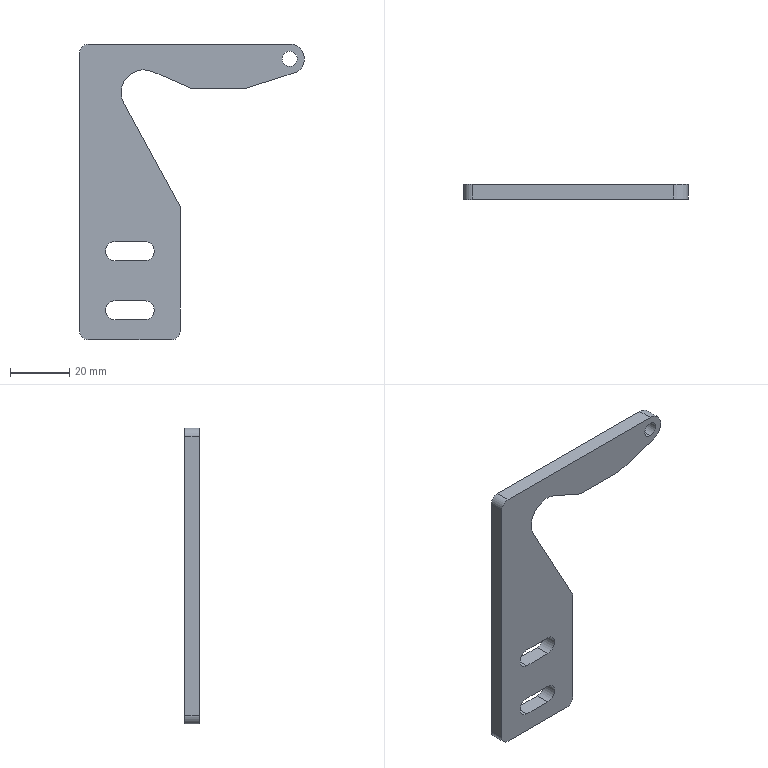Part | SolidWorks | features Extrusion 1, Fillet 1 | 1 solid | 25 faces | box 76 x 5 x 100 mm | volume 16067 mm3 | plane 14 | cylinder 11 | commonest cylinder face diameters 6.5 x4 6 x3 5.2 x2 10 x1 15.307 x1
STEP:
#1=CARTESIAN_POINT('',(54.,5.,82.4));
#2=VERTEX_POINT('',#1);
#3=CARTESIAN_POINT('',(54.,5.,87.6));
#4=VERTEX_POINT('',#3);
#5=CARTESIAN_POINT('',(54.,5.,85.));
#6=DIRECTION('',(0.,1.,0.));
#7=DIRECTION('',(0.,0.,1.));
#8=AXIS2_PLACEMENT_3D('',#5,#6,#7);
#9=CIRCLE('',#8,2.6);
#10=EDGE_CURVE('',#2,#4,#9,.T.);
#11=ORIENTED_EDGE('',*,*,#10,.T.);
#12=CARTESIAN_POINT('',(54.,0.,87.6));
#13=VERTEX_POINT('',#12);
#14=CARTESIAN_POINT('',(54.,5.,87.6));
#15=DIRECTION('',(0.,-1.,0.));
#16=VECTOR('',#15,1000.);
#17=LINE('',#14,#16);
#18=EDGE_CURVE('',#4,#13,#17,.T.);
#19=ORIENTED_EDGE('',*,*,#18,.T.);
#20=CARTESIAN_POINT('',(54.,0.,82.4));
#21=VERTEX_POINT('',#20);
#22=CARTESIAN_POINT('',(54.,0.,85.));
#23=DIRECTION('',(0.,1.,0.));
#24=DIRECTION('',(0.,0.,1.));
#25=AXIS2_PLACEMENT_3D('',#22,#23,#24);
#26=CIRCLE('',#25,2.6);
#27=EDGE_CURVE('',#21,#13,#26,.T.);
#28=ORIENTED_EDGE('',*,*,#27,.F.);
#29=CARTESIAN_POINT('',(54.,5.,82.4));
#30=DIRECTION('',(0.,-1.,0.));
#31=VECTOR('',#30,1000.);
#32=LINE('',#29,#31);
#33=EDGE_CURVE('',#2,#21,#32,.T.);
#34=ORIENTED_EDGE('',*,*,#33,.F.);
#35=EDGE_LOOP('',(#11,#19,#28,#34));
#36=FACE_OUTER_BOUND('',#35,.T.);
#37=CARTESIAN_POINT('',(54.,5.,85.));
#38=DIRECTION('',(0.,-1.,0.));
#39=DIRECTION('',(0.,0.,-1.));
#40=AXIS2_PLACEMENT_3D('',#37,#38,#39);
#41=CYLINDRICAL_SURFACE('',#40,2.6);
#42=ADVANCED_FACE('',(#36),#41,.F.);
#43=CARTESIAN_POINT('',(5.,5.,16.75));
#44=VERTEX_POINT('',#43);
#45=CARTESIAN_POINT('',(-5.,5.,16.75));
#46=VERTEX_POINT('',#45);
#47=CARTESIAN_POINT('',(5.,5.,16.75));
#48=DIRECTION('',(-1.,0.,0.));
#49=VECTOR('',#48,1000.);
#50=LINE('',#47,#49);
#51=EDGE_CURVE('',#44,#46,#50,.T.);
#52=ORIENTED_EDGE('',*,*,#51,.F.);
#53=CARTESIAN_POINT('',(5.,5.,23.25));
#54=VERTEX_POINT('',#53);
#55=CARTESIAN_POINT('',(5.,5.,20.));
#56=DIRECTION('',(0.,1.,0.));
#57=DIRECTION('',(0.,0.,1.));
#58=AXIS2_PLACEMENT_3D('',#55,#56,#57);
#59=CIRCLE('',#58,3.25);
#60=EDGE_CURVE('',#54,#44,#59,.T.);
#61=ORIENTED_EDGE('',*,*,#60,.F.);
#62=CARTESIAN_POINT('',(-5.,5.,23.25));
#63=VERTEX_POINT('',#62);
#64=CARTESIAN_POINT('',(5.,5.,23.25));
#65=DIRECTION('',(1.,0.,0.));
#66=VECTOR('',#65,1000.);
#67=LINE('',#64,#66);
#68=EDGE_CURVE('',#63,#54,#67,.T.);
#69=ORIENTED_EDGE('',*,*,#68,.F.);
#70=CARTESIAN_POINT('',(-5.,5.,20.));
#71=DIRECTION('',(0.,1.,0.));
#72=DIRECTION('',(0.,0.,1.));
#73=AXIS2_PLACEMENT_3D('',#70,#71,#72);
#74=CIRCLE('',#73,3.25);
#75=EDGE_CURVE('',#46,#63,#74,.T.);
#76=ORIENTED_EDGE('',*,*,#75,.F.);
#77=EDGE_LOOP('',(#52,#61,#69,#76));
#78=FACE_BOUND('',#77,.T.);
#79=CARTESIAN_POINT('',(5.,5.,-3.25));
#80=VERTEX_POINT('',#79);
#81=CARTESIAN_POINT('',(-5.,5.,-3.25));
#82=VERTEX_POINT('',#81);
#83=CARTESIAN_POINT('',(5.,5.,-3.25));
#84=DIRECTION('',(-1.,0.,0.));
#85=VECTOR('',#84,1000.);
#86=LINE('',#83,#85);
#87=EDGE_CURVE('',#80,#82,#86,.T.);
#88=ORIENTED_EDGE('',*,*,#87,.F.);
#89=CARTESIAN_POINT('',(5.,5.,3.25));
#90=VERTEX_POINT('',#89);
#91=CARTESIAN_POINT('',(5.,5.,0.));
#92=DIRECTION('',(0.,1.,0.));
#93=DIRECTION('',(0.,0.,1.));
#94=AXIS2_PLACEMENT_3D('',#91,#92,#93);
#95=CIRCLE('',#94,3.25);
#96=EDGE_CURVE('',#90,#80,#95,.T.);
#97=ORIENTED_EDGE('',*,*,#96,.F.);
#98=CARTESIAN_POINT('',(-5.,5.,3.25));
#99=VERTEX_POINT('',#98);
#100=CARTESIAN_POINT('',(5.,5.,3.25));
#101=DIRECTION('',(1.,0.,0.));
#102=VECTOR('',#101,1000.);
#103=LINE('',#100,#102);
#104=EDGE_CURVE('',#99,#90,#103,.T.);
#105=ORIENTED_EDGE('',*,*,#104,.F.);
#106=CARTESIAN_POINT('',(-5.,5.,0.));
#107=DIRECTION('',(0.,1.,0.));
#108=DIRECTION('',(0.,0.,1.));
#109=AXIS2_PLACEMENT_3D('',#106,#107,#108);
#110=CIRCLE('',#109,3.25);
#111=EDGE_CURVE('',#82,#99,#110,.T.);
#112=ORIENTED_EDGE('',*,*,#111,.F.);
#113=EDGE_LOOP('',(#88,#97,#105,#112));
#114=FACE_BOUND('',#113,.T.);
#115=CARTESIAN_POINT('',(14.,5.,-10.));
#116=VERTEX_POINT('',#115);
#117=CARTESIAN_POINT('',(-14.,5.,-10.));
#118=VERTEX_POINT('',#117);
#119=CARTESIAN_POINT('',(-17.,5.,-10.));
#120=DIRECTION('',(-1.,0.,0.));
#121=VECTOR('',#120,1000.);
#122=LINE('',#119,#121);
#123=EDGE_CURVE('',#116,#118,#122,.T.);
#124=ORIENTED_EDGE('',*,*,#123,.T.);
#125=CARTESIAN_POINT('',(-17.,5.,-7.));
#126=VERTEX_POINT('',#125);
#127=CARTESIAN_POINT('',(-14.,5.,-7.));
#128=DIRECTION('',(0.,1.,0.));
#129=DIRECTION('',(0.,0.,1.));
#130=AXIS2_PLACEMENT_3D('',#127,#128,#129);
#131=CIRCLE('',#130,3.);
#132=EDGE_CURVE('',#118,#126,#131,.T.);
#133=ORIENTED_EDGE('',*,*,#132,.T.);
#134=CARTESIAN_POINT('',(-17.,5.,87.));
#135=VERTEX_POINT('',#134);
#136=CARTESIAN_POINT('',(-17.,5.,-10.));
#137=DIRECTION('',(0.,0.,1.));
#138=VECTOR('',#137,1000.);
#139=LINE('',#136,#138);
#140=EDGE_CURVE('',#126,#135,#139,.T.);
#141=ORIENTED_EDGE('',*,*,#140,.T.);
#142=CARTESIAN_POINT('',(-14.,5.,90.));
#143=VERTEX_POINT('',#142);
#144=CARTESIAN_POINT('',(-14.,5.,87.));
#145=DIRECTION('',(0.,1.,0.));
#146=DIRECTION('',(0.,0.,1.));
#147=AXIS2_PLACEMENT_3D('',#144,#145,#146);
#148=CIRCLE('',#147,3.);
#149=EDGE_CURVE('',#135,#143,#148,.T.);
#150=ORIENTED_EDGE('',*,*,#149,.T.);
#151=CARTESIAN_POINT('',(54.,5.,90.));
#152=VERTEX_POINT('',#151);
#153=CARTESIAN_POINT('',(-17.,5.,90.));
#154=DIRECTION('',(1.,0.,0.));
#155=VECTOR('',#154,1000.);
#156=LINE('',#153,#155);
#157=EDGE_CURVE('',#143,#152,#156,.T.);
#158=ORIENTED_EDGE('',*,*,#157,.T.);
#159=CARTESIAN_POINT('',(55.511,5.,80.234));
#160=VERTEX_POINT('',#159);
#161=CARTESIAN_POINT('',(54.,5.,85.));
#162=DIRECTION('',(0.,1.,0.));
#163=DIRECTION('',(0.,0.,1.));
#164=AXIS2_PLACEMENT_3D('',#161,#162,#163);
#165=CIRCLE('',#164,5.);
#166=EDGE_CURVE('',#152,#160,#165,.T.);
#167=ORIENTED_EDGE('',*,*,#166,.T.);
#168=CARTESIAN_POINT('',(39.,5.,75.));
#169=VERTEX_POINT('',#168);
#170=CARTESIAN_POINT('',(39.,5.,75.));
#171=DIRECTION('',(-0.9533,0.,-0.3022));
#172=VECTOR('',#171,1000.);
#173=LINE('',#170,#172);
#174=EDGE_CURVE('',#160,#169,#173,.T.);
#175=ORIENTED_EDGE('',*,*,#174,.T.);
#176=CARTESIAN_POINT('',(20.726,5.,75.));
#177=VERTEX_POINT('',#176);
#178=CARTESIAN_POINT('',(39.,5.,75.));
#179=DIRECTION('',(-1.,0.,0.));
#180=VECTOR('',#179,1000.);
#181=LINE('',#178,#180);
#182=EDGE_CURVE('',#169,#177,#181,.T.);
#183=ORIENTED_EDGE('',*,*,#182,.T.);
#184=CARTESIAN_POINT('',(7.796,5.,80.662));
#185=VERTEX_POINT('',#184);
#186=CARTESIAN_POINT('',(20.726,5.,75.));
#187=DIRECTION('',(-0.916,0.,0.4011));
#188=VECTOR('',#187,1000.);
#189=LINE('',#186,#188);
#190=EDGE_CURVE('',#177,#185,#189,.T.);
#191=ORIENTED_EDGE('',*,*,#190,.T.);
#192=CARTESIAN_POINT('',(-2.,5.,70.));
#193=VERTEX_POINT('',#192);
#194=CARTESIAN_POINT('',(4.726,5.,73.651));
#195=DIRECTION('',(0.,-1.,0.));
#196=DIRECTION('',(0.,0.,1.));
#197=AXIS2_PLACEMENT_3D('',#194,#195,#196);
#198=CIRCLE('',#197,7.653);
#199=EDGE_CURVE('',#185,#193,#198,.T.);
#200=ORIENTED_EDGE('',*,*,#199,.T.);
#201=CARTESIAN_POINT('',(17.,5.,35.));
#202=VERTEX_POINT('',#201);
#203=CARTESIAN_POINT('',(17.,5.,35.));
#204=DIRECTION('',(0.4771,0.,-0.8789));
#205=VECTOR('',#204,1000.);
#206=LINE('',#203,#205);
#207=EDGE_CURVE('',#193,#202,#206,.T.);
#208=ORIENTED_EDGE('',*,*,#207,.T.);
#209=CARTESIAN_POINT('',(17.,5.,-7.));
#210=VERTEX_POINT('',#209);
#211=CARTESIAN_POINT('',(17.,5.,-10.));
#212=DIRECTION('',(0.,0.,-1.));
#213=VECTOR('',#212,1000.);
#214=LINE('',#211,#213);
#215=EDGE_CURVE('',#202,#210,#214,.T.);
#216=ORIENTED_EDGE('',*,*,#215,.T.);
#217=CARTESIAN_POINT('',(14.,5.,-7.));
#218=DIRECTION('',(0.,1.,0.));
#219=DIRECTION('',(0.,0.,1.));
#220=AXIS2_PLACEMENT_3D('',#217,#218,#219);
#221=CIRCLE('',#220,3.);
#222=EDGE_CURVE('',#210,#116,#221,.T.);
#223=ORIENTED_EDGE('',*,*,#222,.T.);
#224=EDGE_LOOP('',(#124,#133,#141,#150,#158,#167,#175,#183,#191,#200,#208,#216,#223));
#225=FACE_OUTER_BOUND('',#224,.T.);
#226=ORIENTED_EDGE('',*,*,#10,.F.);
#227=CARTESIAN_POINT('',(54.,5.,85.));
#228=DIRECTION('',(0.,1.,0.));
#229=DIRECTION('',(0.,0.,1.));
#230=AXIS2_PLACEMENT_3D('',#227,#228,#229);
#231=CIRCLE('',#230,2.6);
#232=EDGE_CURVE('',#4,#2,#231,.T.);
#233=ORIENTED_EDGE('',*,*,#232,.F.);
#234=EDGE_LOOP('',(#226,#233));
#235=FACE_BOUND('',#234,.T.);
#236=CARTESIAN_POINT('',(4.726,5.,73.651));
#237=DIRECTION('',(0.,1.,0.));
#238=DIRECTION('',(0.,0.,1.));
#239=AXIS2_PLACEMENT_3D('',#236,#237,#238);
#240=PLANE('',#239);
#241=ADVANCED_FACE('',(#78,#114,#225,#235),#240,.T.);
#242=CARTESIAN_POINT('',(5.,0.,3.25));
#243=VERTEX_POINT('',#242);
#244=CARTESIAN_POINT('',(5.,0.,-3.25));
#245=VERTEX_POINT('',#244);
#246=CARTESIAN_POINT('',(5.,0.,0.));
#247=DIRECTION('',(0.,1.,0.));
#248=DIRECTION('',(0.,0.,1.));
#249=AXIS2_PLACEMENT_3D('',#246,#247,#248);
#250=CIRCLE('',#249,3.25);
#251=EDGE_CURVE('',#243,#245,#250,.T.);
#252=ORIENTED_EDGE('',*,*,#251,.T.);
#253=CARTESIAN_POINT('',(-5.,0.,-3.25));
#254=VERTEX_POINT('',#253);
#255=CARTESIAN_POINT('',(5.,0.,-3.25));
#256=DIRECTION('',(-1.,0.,0.));
#257=VECTOR('',#256,1000.);
#258=LINE('',#255,#257);
#259=EDGE_CURVE('',#245,#254,#258,.T.);
#260=ORIENTED_EDGE('',*,*,#259,.T.);
#261=CARTESIAN_POINT('',(-5.,0.,3.25));
#262=VERTEX_POINT('',#261);
#263=CARTESIAN_POINT('',(-5.,0.,0.));
#264=DIRECTION('',(0.,1.,0.));
#265=DIRECTION('',(0.,0.,1.));
#266=AXIS2_PLACEMENT_3D('',#263,#264,#265);
#267=CIRCLE('',#266,3.25);
#268=EDGE_CURVE('',#254,#262,#267,.T.);
#269=ORIENTED_EDGE('',*,*,#268,.T.);
#270=CARTESIAN_POINT('',(5.,0.,3.25));
#271=DIRECTION('',(1.,0.,0.));
#272=VECTOR('',#271,1000.);
#273=LINE('',#270,#272);
#274=EDGE_CURVE('',#262,#243,#273,.T.);
#275=ORIENTED_EDGE('',*,*,#274,.T.);
#276=EDGE_LOOP('',(#252,#260,#269,#275));
#277=FACE_BOUND('',#276,.T.);
#278=CARTESIAN_POINT('',(-17.,0.,-7.));
#279=VERTEX_POINT('',#278);
#280=CARTESIAN_POINT('',(-17.,0.,87.));
#281=VERTEX_POINT('',#280);
#282=CARTESIAN_POINT('',(-17.,0.,-10.));
#283=DIRECTION('',(0.,0.,1.));
#284=VECTOR('',#283,1000.);
#285=LINE('',#282,#284);
#286=EDGE_CURVE('',#279,#281,#285,.T.);
#287=ORIENTED_EDGE('',*,*,#286,.F.);
#288=CARTESIAN_POINT('',(-14.,0.,-10.));
#289=VERTEX_POINT('',#288);
#290=CARTESIAN_POINT('',(-14.,0.,-7.));
#291=DIRECTION('',(0.,-1.,0.));
#292=DIRECTION('',(0.,0.,1.));
#293=AXIS2_PLACEMENT_3D('',#290,#291,#292);
#294=CIRCLE('',#293,3.);
#295=EDGE_CURVE('',#279,#289,#294,.T.);
#296=ORIENTED_EDGE('',*,*,#295,.T.);
#297=CARTESIAN_POINT('',(14.,0.,-10.));
#298=VERTEX_POINT('',#297);
#299=CARTESIAN_POINT('',(-17.,0.,-10.));
#300=DIRECTION('',(-1.,0.,0.));
#301=VECTOR('',#300,1000.);
#302=LINE('',#299,#301);
#303=EDGE_CURVE('',#298,#289,#302,.T.);
#304=ORIENTED_EDGE('',*,*,#303,.F.);
#305=CARTESIAN_POINT('',(17.,0.,-7.));
#306=VERTEX_POINT('',#305);
#307=CARTESIAN_POINT('',(14.,0.,-7.));
#308=DIRECTION('',(0.,-1.,0.));
#309=DIRECTION('',(0.,0.,1.));
#310=AXIS2_PLACEMENT_3D('',#307,#308,#309);
#311=CIRCLE('',#310,3.);
#312=EDGE_CURVE('',#298,#306,#311,.T.);
#313=ORIENTED_EDGE('',*,*,#312,.T.);
#314=CARTESIAN_POINT('',(17.,0.,35.));
#315=VERTEX_POINT('',#314);
#316=CARTESIAN_POINT('',(17.,0.,-10.));
#317=DIRECTION('',(0.,0.,-1.));
#318=VECTOR('',#317,1000.);
#319=LINE('',#316,#318);
#320=EDGE_CURVE('',#315,#306,#319,.T.);
#321=ORIENTED_EDGE('',*,*,#320,.F.);
#322=CARTESIAN_POINT('',(-2.,0.,70.));
#323=VERTEX_POINT('',#322);
#324=CARTESIAN_POINT('',(17.,0.,35.));
#325=DIRECTION('',(0.4771,0.,-0.8789));
#326=VECTOR('',#325,1000.);
#327=LINE('',#324,#326);
#328=EDGE_CURVE('',#323,#315,#327,.T.);
#329=ORIENTED_EDGE('',*,*,#328,.F.);
#330=CARTESIAN_POINT('',(7.796,0.,80.662));
#331=VERTEX_POINT('',#330);
#332=CARTESIAN_POINT('',(4.726,0.,73.651));
#333=DIRECTION('',(0.,-1.,0.));
#334=DIRECTION('',(0.,0.,1.));
#335=AXIS2_PLACEMENT_3D('',#332,#333,#334);
#336=CIRCLE('',#335,7.653);
#337=EDGE_CURVE('',#331,#323,#336,.T.);
#338=ORIENTED_EDGE('',*,*,#337,.F.);
#339=CARTESIAN_POINT('',(20.726,0.,75.));
#340=VERTEX_POINT('',#339);
#341=CARTESIAN_POINT('',(20.726,0.,75.));
#342=DIRECTION('',(-0.916,0.,0.4011));
#343=VECTOR('',#342,1000.);
#344=LINE('',#341,#343);
#345=EDGE_CURVE('',#340,#331,#344,.T.);
#346=ORIENTED_EDGE('',*,*,#345,.F.);
#347=CARTESIAN_POINT('',(39.,0.,75.));
#348=VERTEX_POINT('',#347);
#349=CARTESIAN_POINT('',(39.,0.,75.));
#350=DIRECTION('',(-1.,0.,0.));
#351=VECTOR('',#350,1000.);
#352=LINE('',#349,#351);
#353=EDGE_CURVE('',#348,#340,#352,.T.);
#354=ORIENTED_EDGE('',*,*,#353,.F.);
#355=CARTESIAN_POINT('',(55.511,0.,80.234));
#356=VERTEX_POINT('',#355);
#357=CARTESIAN_POINT('',(39.,0.,75.));
#358=DIRECTION('',(-0.9533,0.,-0.3022));
#359=VECTOR('',#358,1000.);
#360=LINE('',#357,#359);
#361=EDGE_CURVE('',#356,#348,#360,.T.);
#362=ORIENTED_EDGE('',*,*,#361,.F.);
#363=CARTESIAN_POINT('',(54.,0.,90.));
#364=VERTEX_POINT('',#363);
#365=CARTESIAN_POINT('',(54.,0.,85.));
#366=DIRECTION('',(0.,1.,0.));
#367=DIRECTION('',(0.,0.,1.));
#368=AXIS2_PLACEMENT_3D('',#365,#366,#367);
#369=CIRCLE('',#368,5.);
#370=EDGE_CURVE('',#364,#356,#369,.T.);
#371=ORIENTED_EDGE('',*,*,#370,.F.);
#372=CARTESIAN_POINT('',(-14.,0.,90.));
#373=VERTEX_POINT('',#372);
#374=CARTESIAN_POINT('',(-17.,0.,90.));
#375=DIRECTION('',(1.,0.,0.));
#376=VECTOR('',#375,1000.);
#377=LINE('',#374,#376);
#378=EDGE_CURVE('',#373,#364,#377,.T.);
#379=ORIENTED_EDGE('',*,*,#378,.F.);
#380=CARTESIAN_POINT('',(-14.,0.,87.));
#381=DIRECTION('',(0.,-1.,0.));
#382=DIRECTION('',(0.,0.,1.));
#383=AXIS2_PLACEMENT_3D('',#380,#381,#382);
#384=CIRCLE('',#383,3.);
#385=EDGE_CURVE('',#373,#281,#384,.T.);
#386=ORIENTED_EDGE('',*,*,#385,.T.);
#387=EDGE_LOOP('',(#287,#296,#304,#313,#321,#329,#338,#346,#354,#362,#371,#379,#386));
#388=FACE_OUTER_BOUND('',#387,.T.);
#389=CARTESIAN_POINT('',(5.,0.,23.25));
#390=VERTEX_POINT('',#389);
#391=CARTESIAN_POINT('',(5.,0.,16.75));
#392=VERTEX_POINT('',#391);
#393=CARTESIAN_POINT('',(5.,0.,20.));
#394=DIRECTION('',(0.,1.,0.));
#395=DIRECTION('',(0.,0.,1.));
#396=AXIS2_PLACEMENT_3D('',#393,#394,#395);
#397=CIRCLE('',#396,3.25);
#398=EDGE_CURVE('',#390,#392,#397,.T.);
#399=ORIENTED_EDGE('',*,*,#398,.T.);
#400=CARTESIAN_POINT('',(-5.,0.,16.75));
#401=VERTEX_POINT('',#400);
#402=CARTESIAN_POINT('',(5.,0.,16.75));
#403=DIRECTION('',(-1.,0.,0.));
#404=VECTOR('',#403,1000.);
#405=LINE('',#402,#404);
#406=EDGE_CURVE('',#392,#401,#405,.T.);
#407=ORIENTED_EDGE('',*,*,#406,.T.);
#408=CARTESIAN_POINT('',(-5.,0.,23.25));
#409=VERTEX_POINT('',#408);
#410=CARTESIAN_POINT('',(-5.,0.,20.));
#411=DIRECTION('',(0.,1.,0.));
#412=DIRECTION('',(0.,0.,1.));
#413=AXIS2_PLACEMENT_3D('',#410,#411,#412);
#414=CIRCLE('',#413,3.25);
#415=EDGE_CURVE('',#401,#409,#414,.T.);
#416=ORIENTED_EDGE('',*,*,#415,.T.);
#417=CARTESIAN_POINT('',(5.,0.,23.25));
#418=DIRECTION('',(1.,0.,0.));
#419=VECTOR('',#418,1000.);
#420=LINE('',#417,#419);
#421=EDGE_CURVE('',#409,#390,#420,.T.);
#422=ORIENTED_EDGE('',*,*,#421,.T.);
#423=EDGE_LOOP('',(#399,#407,#416,#422));
#424=FACE_BOUND('',#423,.T.);
#425=ORIENTED_EDGE('',*,*,#27,.T.);
#426=CARTESIAN_POINT('',(54.,0.,85.));
#427=DIRECTION('',(0.,1.,0.));
#428=DIRECTION('',(0.,0.,1.));
#429=AXIS2_PLACEMENT_3D('',#426,#427,#428);
#430=CIRCLE('',#429,2.6);
#431=EDGE_CURVE('',#13,#21,#430,.T.);
#432=ORIENTED_EDGE('',*,*,#431,.T.);
#433=EDGE_LOOP('',(#425,#432));
#434=FACE_BOUND('',#433,.T.);
#435=CARTESIAN_POINT('',(4.726,0.,73.651));
#436=DIRECTION('',(0.,1.,0.));
#437=DIRECTION('',(0.,0.,1.));
#438=AXIS2_PLACEMENT_3D('',#435,#436,#437);
#439=PLANE('',#438);
#440=ADVANCED_FACE('',(#277,#388,#424,#434),#439,.F.);
#441=ORIENTED_EDGE('',*,*,#303,.T.);
#442=CARTESIAN_POINT('',(-14.,5.,-10.));
#443=DIRECTION('',(0.,1.,0.));
#444=VECTOR('',#443,1000.);
#445=LINE('',#442,#444);
#446=EDGE_CURVE('',#289,#118,#445,.T.);
#447=ORIENTED_EDGE('',*,*,#446,.T.);
#448=ORIENTED_EDGE('',*,*,#123,.F.);
#449=CARTESIAN_POINT('',(14.,5.,-10.));
#450=DIRECTION('',(0.,-1.,0.));
#451=VECTOR('',#450,1000.);
#452=LINE('',#449,#451);
#453=EDGE_CURVE('',#116,#298,#452,.T.);
#454=ORIENTED_EDGE('',*,*,#453,.T.);
#455=EDGE_LOOP('',(#441,#447,#448,#454));
#456=FACE_OUTER_BOUND('',#455,.T.);
#457=CARTESIAN_POINT('',(-17.,5.,-10.));
#458=DIRECTION('',(0.,0.,1.));
#459=DIRECTION('',(1.,0.,0.));
#460=AXIS2_PLACEMENT_3D('',#457,#458,#459);
#461=PLANE('',#460);
#462=ADVANCED_FACE('',(#456),#461,.F.);
#463=ORIENTED_EDGE('',*,*,#140,.F.);
#464=CARTESIAN_POINT('',(-17.,5.,-7.));
#465=DIRECTION('',(0.,-1.,0.));
#466=VECTOR('',#465,1000.);
#467=LINE('',#464,#466);
#468=EDGE_CURVE('',#126,#279,#467,.T.);
#469=ORIENTED_EDGE('',*,*,#468,.T.);
#470=ORIENTED_EDGE('',*,*,#286,.T.);
#471=CARTESIAN_POINT('',(-17.,5.,87.));
#472=DIRECTION('',(0.,1.,0.));
#473=VECTOR('',#472,1000.);
#474=LINE('',#471,#473);
#475=EDGE_CURVE('',#281,#135,#474,.T.);
#476=ORIENTED_EDGE('',*,*,#475,.T.);
#477=EDGE_LOOP('',(#463,#469,#470,#476));
#478=FACE_OUTER_BOUND('',#477,.T.);
#479=CARTESIAN_POINT('',(-17.,5.,-10.));
#480=DIRECTION('',(1.,0.,0.));
#481=DIRECTION('',(0.,0.,-1.));
#482=AXIS2_PLACEMENT_3D('',#479,#480,#481);
#483=PLANE('',#482);
#484=ADVANCED_FACE('',(#478),#483,.F.);
#485=ORIENTED_EDGE('',*,*,#157,.F.);
#486=CARTESIAN_POINT('',(-14.,5.,90.));
#487=DIRECTION('',(0.,-1.,0.));
#488=VECTOR('',#487,1000.);
#489=LINE('',#486,#488);
#490=EDGE_CURVE('',#143,#373,#489,.T.);
#491=ORIENTED_EDGE('',*,*,#490,.T.);
#492=ORIENTED_EDGE('',*,*,#378,.T.);
#493=CARTESIAN_POINT('',(54.,5.,90.));
#494=DIRECTION('',(0.,-1.,0.));
#495=VECTOR('',#494,1000.);
#496=LINE('',#493,#495);
#497=EDGE_CURVE('',#152,#364,#496,.T.);
#498=ORIENTED_EDGE('',*,*,#497,.F.);
#499=EDGE_LOOP('',(#485,#491,#492,#498));
#500=FACE_OUTER_BOUND('',#499,.T.);
#501=CARTESIAN_POINT('',(-17.,5.,90.));
#502=DIRECTION('',(0.,0.,-1.));
#503=DIRECTION('',(-1.,0.,0.));
#504=AXIS2_PLACEMENT_3D('',#501,#502,#503);
#505=PLANE('',#504);
#506=ADVANCED_FACE('',(#500),#505,.F.);
#507=ORIENTED_EDGE('',*,*,#370,.T.);
#508=CARTESIAN_POINT('',(55.511,5.,80.234));
#509=DIRECTION('',(0.,-1.,0.));
#510=VECTOR('',#509,1000.);
#511=LINE('',#508,#510);
#512=EDGE_CURVE('',#160,#356,#511,.T.);
#513=ORIENTED_EDGE('',*,*,#512,.F.);
#514=ORIENTED_EDGE('',*,*,#166,.F.);
#515=ORIENTED_EDGE('',*,*,#497,.T.);
#516=EDGE_LOOP('',(#507,#513,#514,#515));
#517=FACE_OUTER_BOUND('',#516,.T.);
#518=CARTESIAN_POINT('',(54.,5.,85.));
#519=DIRECTION('',(0.,-1.,0.));
#520=DIRECTION('',(0.,0.,-1.));
#521=AXIS2_PLACEMENT_3D('',#518,#519,#520);
#522=CYLINDRICAL_SURFACE('',#521,5.);
#523=ADVANCED_FACE('',(#517),#522,.T.);
#524=ORIENTED_EDGE('',*,*,#361,.T.);
#525=CARTESIAN_POINT('',(39.,5.,75.));
#526=DIRECTION('',(0.,-1.,0.));
#527=VECTOR('',#526,1000.);
#528=LINE('',#525,#527);
#529=EDGE_CURVE('',#169,#348,#528,.T.);
#530=ORIENTED_EDGE('',*,*,#529,.F.);
#531=ORIENTED_EDGE('',*,*,#174,.F.);
#532=ORIENTED_EDGE('',*,*,#512,.T.);
#533=EDGE_LOOP('',(#524,#530,#531,#532));
#534=FACE_OUTER_BOUND('',#533,.T.);
#535=CARTESIAN_POINT('',(39.,5.,75.));
#536=DIRECTION('',(-0.3022,0.,0.9533));
#537=DIRECTION('',(0.9533,0.,0.3022));
#538=AXIS2_PLACEMENT_3D('',#535,#536,#537);
#539=PLANE('',#538);
#540=ADVANCED_FACE('',(#534),#539,.F.);
#541=ORIENTED_EDGE('',*,*,#353,.T.);
#542=CARTESIAN_POINT('',(20.726,5.,75.));
#543=DIRECTION('',(0.,-1.,0.));
#544=VECTOR('',#543,1000.);
#545=LINE('',#542,#544);
#546=EDGE_CURVE('',#177,#340,#545,.T.);
#547=ORIENTED_EDGE('',*,*,#546,.F.);
#548=ORIENTED_EDGE('',*,*,#182,.F.);
#549=ORIENTED_EDGE('',*,*,#529,.T.);
#550=EDGE_LOOP('',(#541,#547,#548,#549));
#551=FACE_OUTER_BOUND('',#550,.T.);
#552=CARTESIAN_POINT('',(39.,5.,75.));
#553=DIRECTION('',(0.,0.,1.));
#554=DIRECTION('',(1.,0.,0.));
#555=AXIS2_PLACEMENT_3D('',#552,#553,#554);
#556=PLANE('',#555);
#557=ADVANCED_FACE('',(#551),#556,.F.);
#558=ORIENTED_EDGE('',*,*,#345,.T.);
#559=CARTESIAN_POINT('',(7.796,5.,80.662));
#560=DIRECTION('',(0.,-1.,0.));
#561=VECTOR('',#560,1000.);
#562=LINE('',#559,#561);
#563=EDGE_CURVE('',#185,#331,#562,.T.);
#564=ORIENTED_EDGE('',*,*,#563,.F.);
#565=ORIENTED_EDGE('',*,*,#190,.F.);
#566=ORIENTED_EDGE('',*,*,#546,.T.);
#567=EDGE_LOOP('',(#558,#564,#565,#566));
#568=FACE_OUTER_BOUND('',#567,.T.);
#569=CARTESIAN_POINT('',(20.726,5.,75.));
#570=DIRECTION('',(0.4011,0.,0.916));
#571=DIRECTION('',(0.916,0.,-0.4011));
#572=AXIS2_PLACEMENT_3D('',#569,#570,#571);
#573=PLANE('',#572);
#574=ADVANCED_FACE('',(#568),#573,.F.);
#575=ORIENTED_EDGE('',*,*,#337,.T.);
#576=CARTESIAN_POINT('',(-2.,5.,70.));
#577=DIRECTION('',(0.,-1.,0.));
#578=VECTOR('',#577,1000.);
#579=LINE('',#576,#578);
#580=EDGE_CURVE('',#193,#323,#579,.T.);
#581=ORIENTED_EDGE('',*,*,#580,.F.);
#582=ORIENTED_EDGE('',*,*,#199,.F.);
#583=ORIENTED_EDGE('',*,*,#563,.T.);
#584=EDGE_LOOP('',(#575,#581,#582,#583));
#585=FACE_OUTER_BOUND('',#584,.T.);
#586=CARTESIAN_POINT('',(4.726,5.,73.651));
#587=DIRECTION('',(0.,-1.,0.));
#588=DIRECTION('',(0.,0.,-1.));
#589=AXIS2_PLACEMENT_3D('',#586,#587,#588);
#590=CYLINDRICAL_SURFACE('',#589,7.653);
#591=ADVANCED_FACE('',(#585),#590,.F.);
#592=ORIENTED_EDGE('',*,*,#328,.T.);
#593=CARTESIAN_POINT('',(17.,5.,35.));
#594=DIRECTION('',(0.,-1.,0.));
#595=VECTOR('',#594,1000.);
#596=LINE('',#593,#595);
#597=EDGE_CURVE('',#202,#315,#596,.T.);
#598=ORIENTED_EDGE('',*,*,#597,.F.);
#599=ORIENTED_EDGE('',*,*,#207,.F.);
#600=ORIENTED_EDGE('',*,*,#580,.T.);
#601=EDGE_LOOP('',(#592,#598,#599,#600));
#602=FACE_OUTER_BOUND('',#601,.T.);
#603=CARTESIAN_POINT('',(17.,5.,35.));
#604=DIRECTION('',(-0.8789,0.,-0.4771));
#605=DIRECTION('',(-0.4771,0.,0.8789));
#606=AXIS2_PLACEMENT_3D('',#603,#604,#605);
#607=PLANE('',#606);
#608=ADVANCED_FACE('',(#602),#607,.F.);
#609=ORIENTED_EDGE('',*,*,#320,.T.);
#610=CARTESIAN_POINT('',(17.,5.,-7.));
#611=DIRECTION('',(0.,1.,0.));
#612=VECTOR('',#611,1000.);
#613=LINE('',#610,#612);
#614=EDGE_CURVE('',#306,#210,#613,.T.);
#615=ORIENTED_EDGE('',*,*,#614,.T.);
#616=ORIENTED_EDGE('',*,*,#215,.F.);
#617=ORIENTED_EDGE('',*,*,#597,.T.);
#618=EDGE_LOOP('',(#609,#615,#616,#617));
#619=FACE_OUTER_BOUND('',#618,.T.);
#620=CARTESIAN_POINT('',(17.,5.,-10.));
#621=DIRECTION('',(-1.,0.,0.));
#622=DIRECTION('',(0.,0.,1.));
#623=AXIS2_PLACEMENT_3D('',#620,#621,#622);
#624=PLANE('',#623);
#625=ADVANCED_FACE('',(#619),#624,.F.);
#626=ORIENTED_EDGE('',*,*,#251,.F.);
#627=CARTESIAN_POINT('',(5.,5.,3.25));
#628=DIRECTION('',(0.,-1.,0.));
#629=VECTOR('',#628,1000.);
#630=LINE('',#627,#629);
#631=EDGE_CURVE('',#90,#243,#630,.T.);
#632=ORIENTED_EDGE('',*,*,#631,.F.);
#633=ORIENTED_EDGE('',*,*,#96,.T.);
#634=CARTESIAN_POINT('',(5.,5.,-3.25));
#635=DIRECTION('',(0.,-1.,0.));
#636=VECTOR('',#635,1000.);
#637=LINE('',#634,#636);
#638=EDGE_CURVE('',#80,#245,#637,.T.);
#639=ORIENTED_EDGE('',*,*,#638,.T.);
#640=EDGE_LOOP('',(#626,#632,#633,#639));
#641=FACE_OUTER_BOUND('',#640,.T.);
#642=CARTESIAN_POINT('',(5.,5.,0.));
#643=DIRECTION('',(0.,-1.,0.));
#644=DIRECTION('',(0.,0.,-1.));
#645=AXIS2_PLACEMENT_3D('',#642,#643,#644);
#646=CYLINDRICAL_SURFACE('',#645,3.25);
#647=ADVANCED_FACE('',(#641),#646,.F.);
#648=ORIENTED_EDGE('',*,*,#259,.F.);
#649=ORIENTED_EDGE('',*,*,#638,.F.);
#650=ORIENTED_EDGE('',*,*,#87,.T.);
#651=CARTESIAN_POINT('',(-5.,5.,-3.25));
#652=DIRECTION('',(0.,-1.,0.));
#653=VECTOR('',#652,1000.);
#654=LINE('',#651,#653);
#655=EDGE_CURVE('',#82,#254,#654,.T.);
#656=ORIENTED_EDGE('',*,*,#655,.T.);
#657=EDGE_LOOP('',(#648,#649,#650,#656));
#658=FACE_OUTER_BOUND('',#657,.T.);
#659=CARTESIAN_POINT('',(5.,5.,-3.25));
#660=DIRECTION('',(0.,0.,1.));
#661=DIRECTION('',(1.,0.,0.));
#662=AXIS2_PLACEMENT_3D('',#659,#660,#661);
#663=PLANE('',#662);
#664=ADVANCED_FACE('',(#658),#663,.T.);
#665=ORIENTED_EDGE('',*,*,#268,.F.);
#666=ORIENTED_EDGE('',*,*,#655,.F.);
#667=ORIENTED_EDGE('',*,*,#111,.T.);
#668=CARTESIAN_POINT('',(-5.,5.,3.25));
#669=DIRECTION('',(0.,-1.,0.));
#670=VECTOR('',#669,1000.);
#671=LINE('',#668,#670);
#672=EDGE_CURVE('',#99,#262,#671,.T.);
#673=ORIENTED_EDGE('',*,*,#672,.T.);
#674=EDGE_LOOP('',(#665,#666,#667,#673));
#675=FACE_OUTER_BOUND('',#674,.T.);
#676=CARTESIAN_POINT('',(-5.,5.,0.));
#677=DIRECTION('',(0.,-1.,0.));
#678=DIRECTION('',(0.,0.,-1.));
#679=AXIS2_PLACEMENT_3D('',#676,#677,#678);
#680=CYLINDRICAL_SURFACE('',#679,3.25);
#681=ADVANCED_FACE('',(#675),#680,.F.);
#682=ORIENTED_EDGE('',*,*,#274,.F.);
#683=ORIENTED_EDGE('',*,*,#672,.F.);
#684=ORIENTED_EDGE('',*,*,#104,.T.);
#685=ORIENTED_EDGE('',*,*,#631,.T.);
#686=EDGE_LOOP('',(#682,#683,#684,#685));
#687=FACE_OUTER_BOUND('',#686,.T.);
#688=CARTESIAN_POINT('',(5.,5.,3.25));
#689=DIRECTION('',(0.,0.,-1.));
#690=DIRECTION('',(-1.,0.,0.));
#691=AXIS2_PLACEMENT_3D('',#688,#689,#690);
#692=PLANE('',#691);
#693=ADVANCED_FACE('',(#687),#692,.T.);
#694=ORIENTED_EDGE('',*,*,#398,.F.);
#695=CARTESIAN_POINT('',(5.,5.,23.25));
#696=DIRECTION('',(0.,-1.,0.));
#697=VECTOR('',#696,1000.);
#698=LINE('',#695,#697);
#699=EDGE_CURVE('',#54,#390,#698,.T.);
#700=ORIENTED_EDGE('',*,*,#699,.F.);
#701=ORIENTED_EDGE('',*,*,#60,.T.);
#702=CARTESIAN_POINT('',(5.,5.,16.75));
#703=DIRECTION('',(0.,-1.,0.));
#704=VECTOR('',#703,1000.);
#705=LINE('',#702,#704);
#706=EDGE_CURVE('',#44,#392,#705,.T.);
#707=ORIENTED_EDGE('',*,*,#706,.T.);
#708=EDGE_LOOP('',(#694,#700,#701,#707));
#709=FACE_OUTER_BOUND('',#708,.T.);
#710=CARTESIAN_POINT('',(5.,5.,20.));
#711=DIRECTION('',(0.,-1.,0.));
#712=DIRECTION('',(0.,0.,-1.));
#713=AXIS2_PLACEMENT_3D('',#710,#711,#712);
#714=CYLINDRICAL_SURFACE('',#713,3.25);
#715=ADVANCED_FACE('',(#709),#714,.F.);
#716=ORIENTED_EDGE('',*,*,#406,.F.);
#717=ORIENTED_EDGE('',*,*,#706,.F.);
#718=ORIENTED_EDGE('',*,*,#51,.T.);
#719=CARTESIAN_POINT('',(-5.,5.,16.75));
#720=DIRECTION('',(0.,-1.,0.));
#721=VECTOR('',#720,1000.);
#722=LINE('',#719,#721);
#723=EDGE_CURVE('',#46,#401,#722,.T.);
#724=ORIENTED_EDGE('',*,*,#723,.T.);
#725=EDGE_LOOP('',(#716,#717,#718,#724));
#726=FACE_OUTER_BOUND('',#725,.T.);
#727=CARTESIAN_POINT('',(5.,5.,16.75));
#728=DIRECTION('',(0.,0.,1.));
#729=DIRECTION('',(1.,0.,0.));
#730=AXIS2_PLACEMENT_3D('',#727,#728,#729);
#731=PLANE('',#730);
#732=ADVANCED_FACE('',(#726),#731,.T.);
#733=ORIENTED_EDGE('',*,*,#415,.F.);
#734=ORIENTED_EDGE('',*,*,#723,.F.);
#735=ORIENTED_EDGE('',*,*,#75,.T.);
#736=CARTESIAN_POINT('',(-5.,5.,23.25));
#737=DIRECTION('',(0.,-1.,0.));
#738=VECTOR('',#737,1000.);
#739=LINE('',#736,#738);
#740=EDGE_CURVE('',#63,#409,#739,.T.);
#741=ORIENTED_EDGE('',*,*,#740,.T.);
#742=EDGE_LOOP('',(#733,#734,#735,#741));
#743=FACE_OUTER_BOUND('',#742,.T.);
#744=CARTESIAN_POINT('',(-5.,5.,20.));
#745=DIRECTION('',(0.,-1.,0.));
#746=DIRECTION('',(0.,0.,-1.));
#747=AXIS2_PLACEMENT_3D('',#744,#745,#746);
#748=CYLINDRICAL_SURFACE('',#747,3.25);
#749=ADVANCED_FACE('',(#743),#748,.F.);
#750=ORIENTED_EDGE('',*,*,#421,.F.);
#751=ORIENTED_EDGE('',*,*,#740,.F.);
#752=ORIENTED_EDGE('',*,*,#68,.T.);
#753=ORIENTED_EDGE('',*,*,#699,.T.);
#754=EDGE_LOOP('',(#750,#751,#752,#753));
#755=FACE_OUTER_BOUND('',#754,.T.);
#756=CARTESIAN_POINT('',(5.,5.,23.25));
#757=DIRECTION('',(0.,0.,-1.));
#758=DIRECTION('',(-1.,0.,0.));
#759=AXIS2_PLACEMENT_3D('',#756,#757,#758);
#760=PLANE('',#759);
#761=ADVANCED_FACE('',(#755),#760,.T.);
#762=ORIENTED_EDGE('',*,*,#18,.F.);
#763=ORIENTED_EDGE('',*,*,#232,.T.);
#764=ORIENTED_EDGE('',*,*,#33,.T.);
#765=ORIENTED_EDGE('',*,*,#431,.F.);
#766=EDGE_LOOP('',(#762,#763,#764,#765));
#767=FACE_OUTER_BOUND('',#766,.T.);
#768=CARTESIAN_POINT('',(54.,5.,85.));
#769=DIRECTION('',(0.,-1.,0.));
#770=DIRECTION('',(0.,0.,-1.));
#771=AXIS2_PLACEMENT_3D('',#768,#769,#770);
#772=CYLINDRICAL_SURFACE('',#771,2.6);
#773=ADVANCED_FACE('',(#767),#772,.F.);
#774=ORIENTED_EDGE('',*,*,#132,.F.);
#775=ORIENTED_EDGE('',*,*,#446,.F.);
#776=ORIENTED_EDGE('',*,*,#295,.F.);
#777=ORIENTED_EDGE('',*,*,#468,.F.);
#778=EDGE_LOOP('',(#774,#775,#776,#777));
#779=FACE_OUTER_BOUND('',#778,.T.);
#780=CARTESIAN_POINT('',(-14.,5.,-7.));
#781=DIRECTION('',(0.,-1.,0.));
#782=DIRECTION('',(0.,0.,-1.));
#783=AXIS2_PLACEMENT_3D('',#780,#781,#782);
#784=CYLINDRICAL_SURFACE('',#783,3.);
#785=ADVANCED_FACE('',(#779),#784,.T.);
#786=ORIENTED_EDGE('',*,*,#222,.F.);
#787=ORIENTED_EDGE('',*,*,#614,.F.);
#788=ORIENTED_EDGE('',*,*,#312,.F.);
#789=ORIENTED_EDGE('',*,*,#453,.F.);
#790=EDGE_LOOP('',(#786,#787,#788,#789));
#791=FACE_OUTER_BOUND('',#790,.T.);
#792=CARTESIAN_POINT('',(14.,5.,-7.));
#793=DIRECTION('',(0.,-1.,0.));
#794=DIRECTION('',(0.,0.,-1.));
#795=AXIS2_PLACEMENT_3D('',#792,#793,#794);
#796=CYLINDRICAL_SURFACE('',#795,3.);
#797=ADVANCED_FACE('',(#791),#796,.T.);
#798=ORIENTED_EDGE('',*,*,#149,.F.);
#799=ORIENTED_EDGE('',*,*,#475,.F.);
#800=ORIENTED_EDGE('',*,*,#385,.F.);
#801=ORIENTED_EDGE('',*,*,#490,.F.);
#802=EDGE_LOOP('',(#798,#799,#800,#801));
#803=FACE_OUTER_BOUND('',#802,.T.);
#804=CARTESIAN_POINT('',(-14.,5.,87.));
#805=DIRECTION('',(0.,-1.,0.));
#806=DIRECTION('',(0.,0.,-1.));
#807=AXIS2_PLACEMENT_3D('',#804,#805,#806);
#808=CYLINDRICAL_SURFACE('',#807,3.);
#809=ADVANCED_FACE('',(#803),#808,.T.);
#810=CLOSED_SHELL('',(#42,#241,#440,#462,#484,#506,#523,#540,#557,#574,#591,#608,#625,#647,#664,#681,#693,#715,#732,#749,#761,#773,#785,#797,#809));
#811=MANIFOLD_SOLID_BREP('',#810);
#812=CARTESIAN_POINT('',(0.,0.,0.));
#813=DIRECTION('',(0.,0.,1.));
#814=DIRECTION('',(1.,0.,0.));
#815=AXIS2_PLACEMENT_3D('',#812,#813,#814);
#816=(LENGTH_UNIT()NAMED_UNIT(*)SI_UNIT(.MILLI.,.METRE.));
#817=UNCERTAINTY_MEASURE_WITH_UNIT(LENGTH_MEASURE(0.00001),#816,'','');
#818=(NAMED_UNIT(*)PLANE_ANGLE_UNIT()SI_UNIT($,.RADIAN.));
#819=(NAMED_UNIT(*)SI_UNIT($,.STERADIAN.)SOLID_ANGLE_UNIT());
#820=(GEOMETRIC_REPRESENTATION_CONTEXT(3)GLOBAL_UNCERTAINTY_ASSIGNED_CONTEXT((#817))GLOBAL_UNIT_ASSIGNED_CONTEXT((#816,#818,#819))REPRESENTATION_CONTEXT('',''));
#821=ADVANCED_BREP_SHAPE_REPRESENTATION('',(#811,#815),#820);